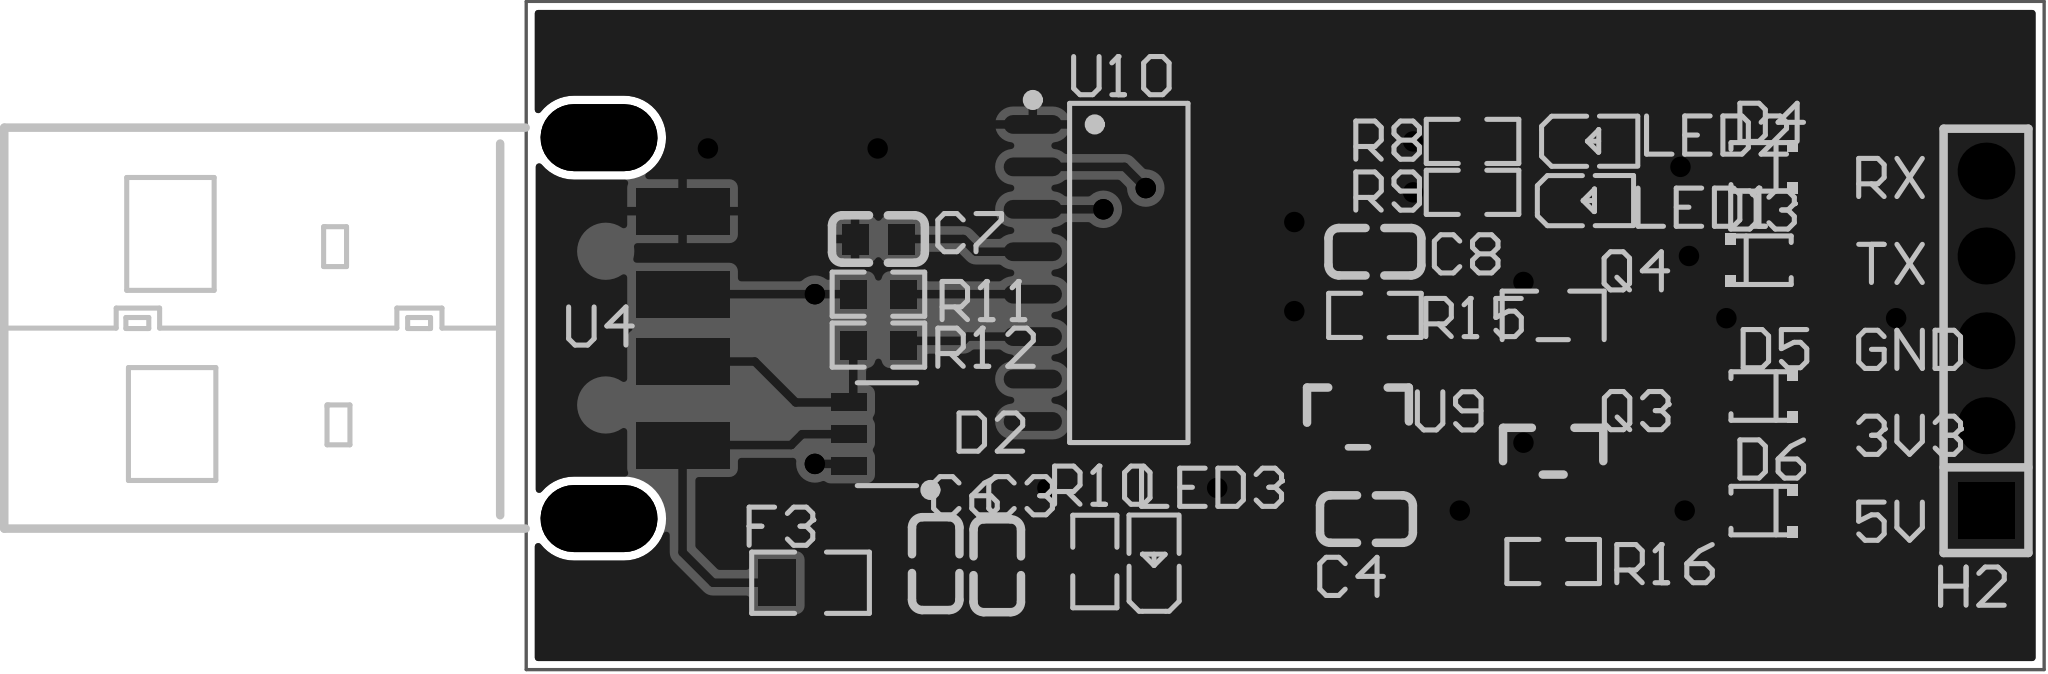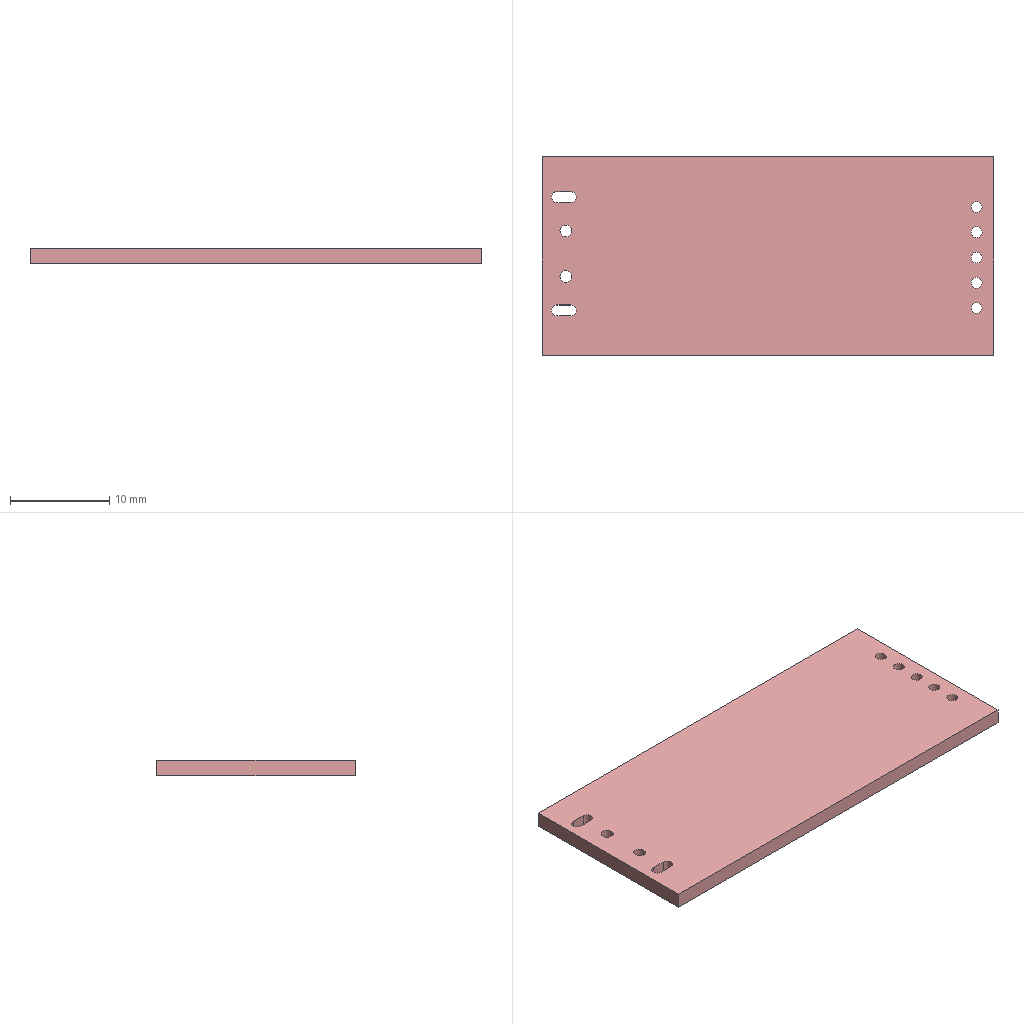Circuit board layout | Altium Designer | box 45.4 x 20 x 1.6 mm
Layer stack:
# Altium Designer layer stack of  (unit mm; dielectric type: 0 none, 1 core, 2 prepreg, 3 surface material)
index,name,kind,layer,copper_thickness_mm,dielectric_type,dielectric_thickness_mm,dielectric_material,dielectric_constant
0,Top Paste Mask Layer,other,,,,,,
1,Top Silkscreen Layer,other,,,,,,
2,Top Solder Mask Layer,dielectric,,,3,0.01,,3.3
3,Top Layer,copper,Top Layer,0.035,,,,
4,Dielectric1,dielectric,,,3,1.51,FR4,4.5
5,Bottom Layer,copper,Bottom Layer,0.035,,,,
6,Bottom Solder Mask Layer,dielectric,,,3,0.01,,3.3
7,Bottom Silkscreen Layer,other,,,,,,
8,Bottom Paste Mask Layer,other,,,,,,
# drill layer pairs: low layer,high layer
drill_pair,Top Layer,Bottom Layer
Part placement:
Designator,Comment,Layer,Footprint,Center-X(mm),Center-Y(mm),Rotation
C3,100nF,TopLayer,C0603,105.918,79.309,90
C4,100nF,TopLayer,C0603,116.967,80.706,0
C6,100nF,TopLayer,C0603,104.077,79.373,270
C7,100nF,TopLayer,C0603,102.362,89.088,180
C8,10uF,TopLayer,C0603,117.221,88.707,180
D2,USBLC6-2SC6,TopLayer,SOT-23-6_L2.9-W1.6-P0.95-LS2.8-BL,102.616,83.246,90
D3,1N5819WS,TopLayer,SOD-323_L1.8-W1.3-LS2.5-RD,128.778,88.453,0
D4,1N5819WS,TopLayer,SOD-323_L1.8-W1.3-LS2.5-RD,128.778,91.247,180
D5,1N5819WS,TopLayer,SOD-323_L1.8-W1.3-LS2.5-RD,128.778,84.389,180
D6,1N5819WS,TopLayer,SOD-323_L1.8-W1.3-LS2.5-RD,128.778,80.96,180
F3,SMD0805-100-12,TopLayer,R0805,100.33,78.801,0
H2,PZ254V-11-05P,TopLayer,HDR-TH_5P-P2.54-V-M,135.509,86.04,90
LED1,MHT192DUGCT,TopLayer,LED0603-RD,123.571,90.231,0
LED2,LTST-C193KRKT-5A,TopLayer,LED0603-RD,123.698,92.009,0
LED3,MHT192DUGCT,TopLayer,LED0603-RD,110.617,79.436,90
Q3,AO3401A,TopLayer,SOT-23_L2.9-W1.3-P1.90-LS2.4-BR,122.555,82.738,270
Q4,S8050-J3Y,TopLayer,SOT-23-3_L2.9-W1.3-P0.95-LS2.4-BR-1,122.555,86.802,270
R8,1kΩ,TopLayer,R0603,120.142,92.009,0
R9,1kΩ,TopLayer,R0603,120.142,90.485,0
R10,10kΩ,TopLayer,R0603,108.839,79.436,270
R11,33kΩ,TopLayer,R0603,102.362,87.437,0
R12,33kΩ,TopLayer,R0603,102.362,85.913,0
R15,10kΩ,TopLayer,R0603,117.221,86.802,180
R16,10kΩ,TopLayer,R0603,122.555,79.436,0
U4,KH-USB180-AM-4P,TopLayer,USB-A-SMD_USB-A-1-TH,95.25,86.421,180
U10,CH340C,TopLayer,SOP-16_L10.0-W3.9-P1.27-LS6.0-BL,109.855,88.072,270
U9,XC6206-3.3V,TopLayer,SSOT-3_L2.9-W1.6-P0.95-LS2.8-BR,116.713,83.754,270
Pad and via stacks:
# Altium Designer via and pad stacks of  (unit mm). Each distinct definition once, with the count of objects using it.
# via: kind,start_layer,end_layer,hole_mm,diameter_mm,mode(0 simple;1 top-mid-bottom;2 full stack),diameter_per_layer,count,example_net
# pad: kind,layer,hole_mm,hole_type(0 round;1 square;2 slot),plating,top_size,top_shape(1 round;2 rect;3 octagon;9 rounded rect),mid_size,bottom_size,mode,footprint,size_per_layer,count,example
pad,Top Layer,0,0,plated,0.8x0.9,2,0.8x0.9,0.8x0.9,0,C0603,,10,C3.2
pad,Top Layer,0,0,plated,0.532x1.072,2,0.532x1.072,0.532x1.072,0,SOT-23-6_L2.9-W1.6-P0.95-LS2.8-BL,,6,D2.1
pad,Top Layer,0,0,plated,1x0.75,2,1x0.75,1x0.75,0,SOD-323_L1.8-W1.3-LS2.5-RD,,8,D3.2
pad,Top Layer,0,0,plated,1.133x1.377,2,1.133x1.377,1.133x1.377,0,R0805,,2,F3.2
pad,Top Layer,0,0,plated,0.8x0.8,2,0.8x0.8,0.8x0.8,0,LED0603-RD,,6,LED1.2
pad,Top Layer,0,0,plated,1x0.8,2,1x0.8,1x0.8,0,SOT-23_L2.9-W1.3-P1.90-LS2.4-BR,,3,Q3.2
pad,Top Layer,0,0,plated,1.25x0.7,2,1.25x0.7,1.25x0.7,0,SOT-23-3_L2.9-W1.3-P0.95-LS2.4-BR-1,,3,Q4.1
pad,Top Layer,0,0,plated,0.8065x0.864,2,0.8065x0.864,0.8065x0.864,0,R0603,,14,R8.2
pad,Top Layer,0,0,plated,2.8x1.4,2,2.8x1.4,2.8x1.4,0,USB-A-SMD_USB-A-1-TH,,4,U4.3
pad,Top Layer,0,0,plated,0.56x1.745,1,0.56x1.745,0.56x1.745,0,SOP-16_L10.0-W3.9-P1.27-LS6.0-BL,,16,U10.1
pad,Top Layer,0,0,plated,0.8x1,2,0.8x1,0.8x1,0,SSOT-3_L2.9-W1.6-P0.95-LS2.8-BR,,3,U9.3
pad,Multi-Layer,1.1,0,plated,1.7x1.7,2,1.7x1.7,1.7x1.7,0,HDR-TH_5P-P2.54-V-M,,1,H2.1
pad,Multi-Layer,1.1,0,plated,1.7x1.7,1,1.7x1.7,1.7x1.7,0,HDR-TH_5P-P2.54-V-M,,4,H2.2
pad,Multi-Layer,1.1,2,plated,3.5x2,1,3.5x2,3.5x2,0,USB-A-SMD_USB-A-1-TH,,2,U4.5
via,Top Layer,Bottom Layer,0.3048,0.61,0,,20,$1N44
Copper pours:
name,layer,net,type(0 solid;1 hatched;2 none)
Top Layer-GND,Top Layer,GND,0
Bottom Layer-GND,Bottom Layer,GND,0
Design rules, without the lines most boards share:
# Altium Designer design rules of  (exported by Altium Designer, unit mm)
# columns: name | kind | enabled | priority | scope1 | scope2 | descriptor | typed fields (field=value)
Copper_copperRegion_copperThickness1oz | 0 | disabled | 4 | All | All | Clearance Constraint (Gap=5.984mil) (Disabled)(All),(All) | gap=0.152
Copper_copperRegion_copperThickness1oz_1 | 63 | disabled | 4 | All | All | Board Clearance Constraint (Gap=0mil) (Disabled)(All) |
Copper_copperRegion_Copper_copperRegion | 0 | disabled | 5 | All | All | Clearance Constraint (Gap=5.984mil) (Disabled)(All),(All) | gap=0.152
Copper_copperRegion_Copper_copperRegion_1 | 63 | disabled | 5 | All | All | Board Clearance Constraint (Gap=0mil) (Disabled)(All) |
copperThickness1oz | 0 | enabled | 6 | All | All | Clearance Constraint (Gap=5.984mil) (All),(All) | gap=0.152
copperThickness1oz_1 | 63 | enabled | 6 | All | All | Board Clearance Constraint (Gap=0mil) (All) |
copperRegion_copperThickness1oz | 20 | disabled | 1 | All | All | Polygon Connect Rule(Relief Connect )(Conductor Width=10mil) (Relief Angle=90 Angle) (Entries=4) (Air Gap Width=10mil) (Disabled)(All),(All) | connect_style(0=relief,1=direct,2=none)=0 relief_conductor_width=0.254 relief_entries=4
copperRegion_Copper_copperRegion | 20 | disabled | 2 | All | All | Polygon Connect Rule(Relief Connect )(Conductor Width=10mil) (Relief Angle=90 Angle) (Entries=4) (Air Gap Width=10mil) (Disabled)(All),(All) | connect_style(0=relief,1=direct,2=none)=0 relief_conductor_width=0.254 relief_entries=4
copperRegion | 20 | enabled | 3 | All | All | Polygon Connect Rule(Relief Connect )(Conductor Width=10mil) (Relief Angle=90 Angle) (Entries=4) (Air Gap Width=10mil) (All),(All) | connect_style(0=relief,1=direct,2=none)=0 relief_conductor_width=0.254 relief_entries=4